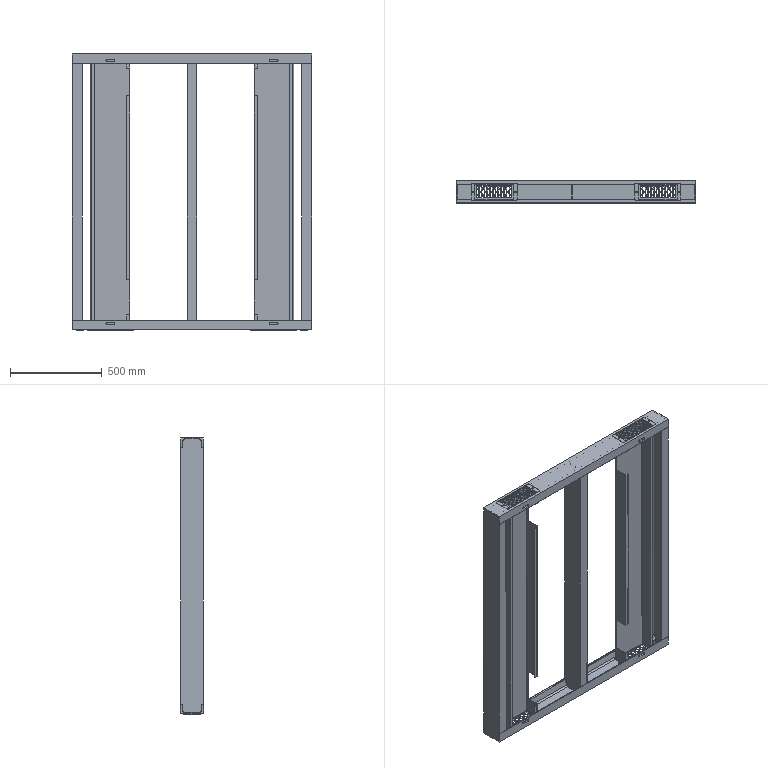Part | SolidWorks | 15 solids | 1044 faces | box 1300 x 120 x 1504 mm | volume 13170720 mm3 | plane 678 | cylinder 366 | commonest cylinder face diameters 12 x208 10 x32 6 x28 2 x16 5 x16 5.5 x16